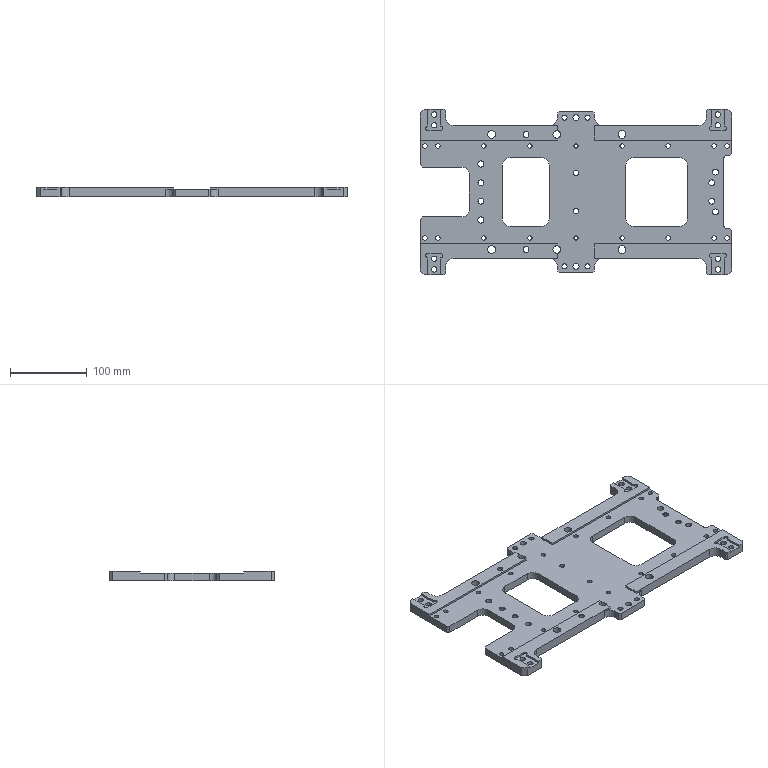Part | STEP file | J454-EBZ05-06-00-Part-1 | 1 solid | 276 faces | box 406 x 216 x 12.5 mm | volume 586432 mm3 | cylinder 172 | plane 104 | commonest cylinder face diameters 8 x24 6 x20 20 x18 5.5 x16 7 x16 9.5 x16